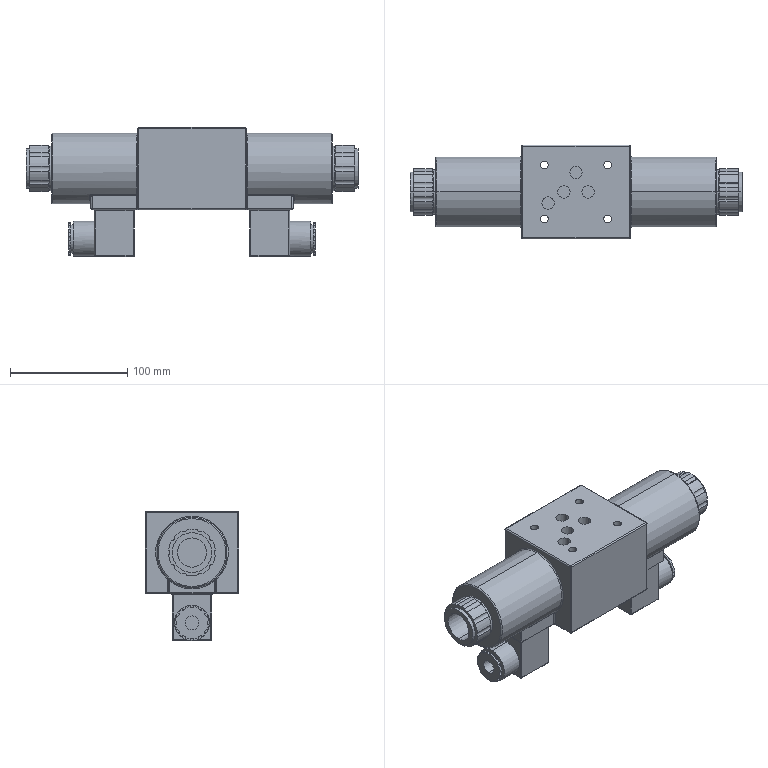Part | SolidWorks | features ICE 10, Extrusion 1, Fillet 1, MirrorPattern 1, Revolution 1 | 1 solid | 331 faces | box 283 x 80 x 110 mm | volume 1025505 mm3 | cylinder 210 | plane 46 | sphere 24 | cone 22 | torus 21 | spline 8 | commonest cylinder face diameters 2 x58 4 x30 6 x24 28 x24 40 x22 6.7 x8